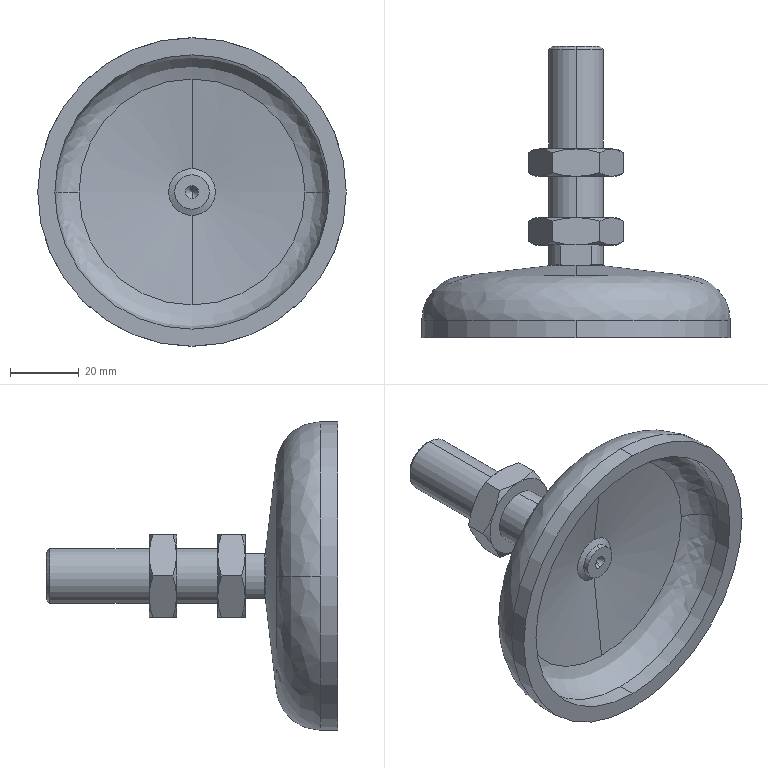Part | STEP file | 1 solid | 85 faces | box 90 x 85 x 90 mm | volume 60517 mm3 | cone 32 | plane 25 | cylinder 19 | spline 9 | commonest cylinder face diameters 16 x9 7.5 x2 8 x2 10 x2 80 x2 90 x2